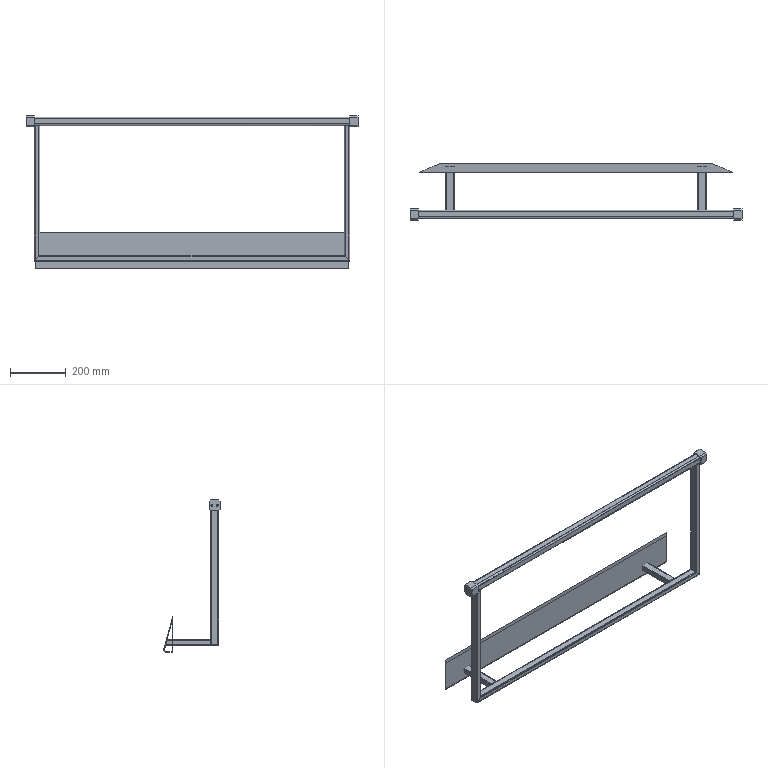Part | SolidWorks | features ICE 7, 3DProfileFeature 4, HoleWzd 2, WeldMemberFeat 2, MirrorPattern 1, WeldmentFeature 1 | 7 solids | 164 faces | box 1194 x 202.556 x 548 mm | volume 1440034 mm3 | plane 92 | cylinder 68 | cone 4 | commonest cylinder face diameters 4 x12 6 x12 8 x12 2 x8 5 x8 6.8 x8